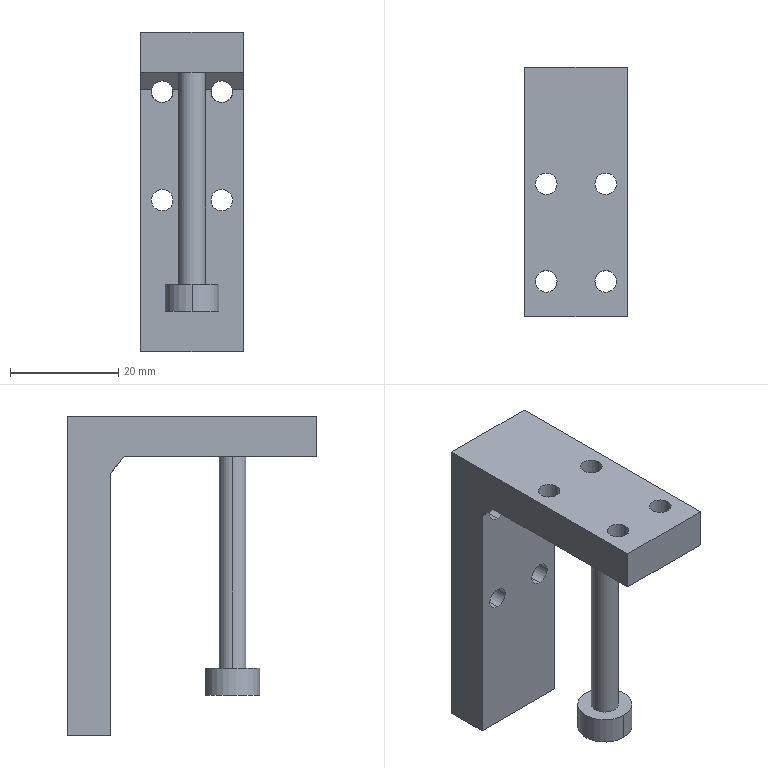Part | NX | 1 solid | 31 faces | box 19 x 46 x 59 mm | volume 14830 mm3 | cylinder 20 | plane 11 | commonest cylinder face diameters 4 x16 5 x2 10 x2
STEP:
#1=CARTESIAN_POINT('',(0.,5.,-51.5));
#2=VERTEX_POINT('',#1);
#3=CARTESIAN_POINT('',(0.,-5.,-51.5));
#4=VERTEX_POINT('',#3);
#5=CARTESIAN_POINT('',(0.,0.,-51.5));
#6=DIRECTION('',(0.,0.,-1.));
#7=DIRECTION('',(0.,1.,0.));
#8=AXIS2_PLACEMENT_3D('',#5,#6,#7);
#9=CIRCLE('',#8,5.);
#10=EDGE_CURVE('',#2,#4,#9,.T.);
#11=ORIENTED_EDGE('',*,*,#10,.F.);
#12=CARTESIAN_POINT('',(0.,5.,-46.5));
#13=VERTEX_POINT('',#12);
#14=CARTESIAN_POINT('',(0.,5.,-51.5));
#15=DIRECTION('',(0.,0.,1.));
#16=VECTOR('',#15,1000.);
#17=LINE('',#14,#16);
#18=EDGE_CURVE('',#2,#13,#17,.T.);
#19=ORIENTED_EDGE('',*,*,#18,.T.);
#20=CARTESIAN_POINT('',(0.,-5.,-46.5));
#21=VERTEX_POINT('',#20);
#22=CARTESIAN_POINT('',(0.,0.,-46.5));
#23=DIRECTION('',(0.,0.,-1.));
#24=DIRECTION('',(0.,1.,0.));
#25=AXIS2_PLACEMENT_3D('',#22,#23,#24);
#26=CIRCLE('',#25,5.);
#27=EDGE_CURVE('',#13,#21,#26,.T.);
#28=ORIENTED_EDGE('',*,*,#27,.T.);
#29=CARTESIAN_POINT('',(0.,-5.,-51.5));
#30=DIRECTION('',(0.,0.,1.));
#31=VECTOR('',#30,1000.);
#32=LINE('',#29,#31);
#33=EDGE_CURVE('',#4,#21,#32,.T.);
#34=ORIENTED_EDGE('',*,*,#33,.F.);
#35=EDGE_LOOP('',(#11,#19,#28,#34));
#36=FACE_BOUND('',#35,.T.);
#37=CARTESIAN_POINT('',(0.,0.,-51.5));
#38=DIRECTION('',(0.,0.,1.));
#39=DIRECTION('',(0.,-1.,0.));
#40=AXIS2_PLACEMENT_3D('',#37,#38,#39);
#41=CYLINDRICAL_SURFACE('',#40,5.);
#42=ADVANCED_FACE('',(#36),#41,.T.);
#43=CARTESIAN_POINT('',(5.5,22.5,-13.));
#44=VERTEX_POINT('',#43);
#45=CARTESIAN_POINT('',(3.564,22.5,-10.5));
#46=VERTEX_POINT('',#45);
#47=CARTESIAN_POINT('',(5.5,22.5,-11.));
#48=DIRECTION('',(0.,1.,0.));
#49=DIRECTION('',(0.,0.,1.));
#50=AXIS2_PLACEMENT_3D('',#47,#48,#49);
#51=CIRCLE('',#50,2.);
#52=EDGE_CURVE('',#44,#46,#51,.T.);
#53=ORIENTED_EDGE('',*,*,#52,.F.);
#54=CARTESIAN_POINT('',(5.5,30.5,-13.));
#55=VERTEX_POINT('',#54);
#56=CARTESIAN_POINT('',(5.5,-15.5,-13.));
#57=DIRECTION('',(0.,1.,0.));
#58=VECTOR('',#57,1000.);
#59=LINE('',#56,#58);
#60=EDGE_CURVE('',#44,#55,#59,.T.);
#61=ORIENTED_EDGE('',*,*,#60,.T.);
#62=CARTESIAN_POINT('',(5.5,30.5,-9.));
#63=VERTEX_POINT('',#62);
#64=CARTESIAN_POINT('',(5.5,30.5,-11.));
#65=DIRECTION('',(0.,1.,0.));
#66=DIRECTION('',(0.,0.,-1.));
#67=AXIS2_PLACEMENT_3D('',#64,#65,#66);
#68=CIRCLE('',#67,2.);
#69=EDGE_CURVE('',#55,#63,#68,.T.);
#70=ORIENTED_EDGE('',*,*,#69,.T.);
#71=CARTESIAN_POINT('',(5.5,21.241,-9.));
#72=VERTEX_POINT('',#71);
#73=CARTESIAN_POINT('',(5.5,-15.5,-9.));
#74=DIRECTION('',(0.,1.,0.));
#75=VECTOR('',#74,1000.);
#76=LINE('',#73,#75);
#77=EDGE_CURVE('',#72,#63,#76,.T.);
#78=ORIENTED_EDGE('',*,*,#77,.F.);
#79=CARTESIAN_POINT('',(3.564,22.5,-10.5));
#80=CARTESIAN_POINT('',(3.801,21.729,-9.581));
#81=CARTESIAN_POINT('',(4.551,21.241,-9.));
#82=CARTESIAN_POINT('',(5.5,21.241,-9.));
#83=(BOUNDED_CURVE()B_SPLINE_CURVE(3,(#79,#80,#81,#82),.UNSPECIFIED.,.F.,.F.)B_SPLINE_CURVE_WITH_KNOTS((4,4),(1.823,3.142),.UNSPECIFIED.)CURVE()GEOMETRIC_REPRESENTATION_ITEM()RATIONAL_B_SPLINE_CURVE((1.,0.8604,0.8604,1.))REPRESENTATION_ITEM(''));
#84=EDGE_CURVE('',#46,#72,#83,.T.);
#85=ORIENTED_EDGE('',*,*,#84,.F.);
#86=EDGE_LOOP('',(#53,#61,#70,#78,#85));
#87=FACE_BOUND('',#86,.T.);
#88=CARTESIAN_POINT('',(5.5,-15.5,-11.));
#89=DIRECTION('',(0.,1.,0.));
#90=DIRECTION('',(0.,0.,1.));
#91=AXIS2_PLACEMENT_3D('',#88,#89,#90);
#92=CYLINDRICAL_SURFACE('',#91,2.);
#93=ADVANCED_FACE('',(#87),#92,.F.);
#94=CARTESIAN_POINT('',(-5.5,22.5,-29.));
#95=VERTEX_POINT('',#94);
#96=CARTESIAN_POINT('',(-5.5,22.5,-33.));
#97=VERTEX_POINT('',#96);
#98=CARTESIAN_POINT('',(-5.5,22.5,-31.));
#99=DIRECTION('',(0.,1.,0.));
#100=DIRECTION('',(0.,0.,1.));
#101=AXIS2_PLACEMENT_3D('',#98,#99,#100);
#102=CIRCLE('',#101,2.);
#103=EDGE_CURVE('',#95,#97,#102,.T.);
#104=ORIENTED_EDGE('',*,*,#103,.F.);
#105=CARTESIAN_POINT('',(-5.5,30.5,-29.));
#106=VERTEX_POINT('',#105);
#107=CARTESIAN_POINT('',(-5.5,-15.5,-29.));
#108=DIRECTION('',(0.,1.,0.));
#109=VECTOR('',#108,1000.);
#110=LINE('',#107,#109);
#111=EDGE_CURVE('',#95,#106,#110,.T.);
#112=ORIENTED_EDGE('',*,*,#111,.T.);
#113=CARTESIAN_POINT('',(-5.5,30.5,-33.));
#114=VERTEX_POINT('',#113);
#115=CARTESIAN_POINT('',(-5.5,30.5,-31.));
#116=DIRECTION('',(0.,1.,0.));
#117=DIRECTION('',(0.,0.,1.));
#118=AXIS2_PLACEMENT_3D('',#115,#116,#117);
#119=CIRCLE('',#118,2.);
#120=EDGE_CURVE('',#106,#114,#119,.T.);
#121=ORIENTED_EDGE('',*,*,#120,.T.);
#122=CARTESIAN_POINT('',(-5.5,-15.5,-33.));
#123=DIRECTION('',(0.,1.,0.));
#124=VECTOR('',#123,1000.);
#125=LINE('',#122,#124);
#126=EDGE_CURVE('',#97,#114,#125,.T.);
#127=ORIENTED_EDGE('',*,*,#126,.F.);
#128=EDGE_LOOP('',(#104,#112,#121,#127));
#129=FACE_BOUND('',#128,.T.);
#130=CARTESIAN_POINT('',(-5.5,-15.5,-31.));
#131=DIRECTION('',(0.,1.,0.));
#132=DIRECTION('',(0.,0.,1.));
#133=AXIS2_PLACEMENT_3D('',#130,#131,#132);
#134=CYLINDRICAL_SURFACE('',#133,2.);
#135=ADVANCED_FACE('',(#129),#134,.F.);
#136=CARTESIAN_POINT('',(-5.5,22.5,-13.));
#137=VERTEX_POINT('',#136);
#138=CARTESIAN_POINT('',(-7.436,22.5,-10.5));
#139=VERTEX_POINT('',#138);
#140=CARTESIAN_POINT('',(-5.5,22.5,-11.));
#141=DIRECTION('',(0.,1.,0.));
#142=DIRECTION('',(0.,0.,1.));
#143=AXIS2_PLACEMENT_3D('',#140,#141,#142);
#144=CIRCLE('',#143,2.);
#145=EDGE_CURVE('',#137,#139,#144,.T.);
#146=ORIENTED_EDGE('',*,*,#145,.F.);
#147=CARTESIAN_POINT('',(-5.5,30.5,-13.));
#148=VERTEX_POINT('',#147);
#149=CARTESIAN_POINT('',(-5.5,-15.5,-13.));
#150=DIRECTION('',(0.,1.,0.));
#151=VECTOR('',#150,1000.);
#152=LINE('',#149,#151);
#153=EDGE_CURVE('',#137,#148,#152,.T.);
#154=ORIENTED_EDGE('',*,*,#153,.T.);
#155=CARTESIAN_POINT('',(-5.5,30.5,-9.));
#156=VERTEX_POINT('',#155);
#157=CARTESIAN_POINT('',(-5.5,30.5,-11.));
#158=DIRECTION('',(0.,1.,0.));
#159=DIRECTION('',(0.,0.,1.));
#160=AXIS2_PLACEMENT_3D('',#157,#158,#159);
#161=CIRCLE('',#160,2.);
#162=EDGE_CURVE('',#148,#156,#161,.T.);
#163=ORIENTED_EDGE('',*,*,#162,.T.);
#164=CARTESIAN_POINT('',(-5.5,21.241,-9.));
#165=VERTEX_POINT('',#164);
#166=CARTESIAN_POINT('',(-5.5,-15.5,-9.));
#167=DIRECTION('',(0.,1.,0.));
#168=VECTOR('',#167,1000.);
#169=LINE('',#166,#168);
#170=EDGE_CURVE('',#165,#156,#169,.T.);
#171=ORIENTED_EDGE('',*,*,#170,.F.);
#172=CARTESIAN_POINT('',(-7.436,22.5,-10.5));
#173=CARTESIAN_POINT('',(-7.199,21.729,-9.581));
#174=CARTESIAN_POINT('',(-6.449,21.241,-9.));
#175=CARTESIAN_POINT('',(-5.5,21.241,-9.));
#176=(BOUNDED_CURVE()B_SPLINE_CURVE(3,(#172,#173,#174,#175),.UNSPECIFIED.,.F.,.F.)B_SPLINE_CURVE_WITH_KNOTS((4,4),(1.823,3.142),.UNSPECIFIED.)CURVE()GEOMETRIC_REPRESENTATION_ITEM()RATIONAL_B_SPLINE_CURVE((1.,0.8604,0.8604,1.))REPRESENTATION_ITEM(''));
#177=EDGE_CURVE('',#139,#165,#176,.T.);
#178=ORIENTED_EDGE('',*,*,#177,.F.);
#179=EDGE_LOOP('',(#146,#154,#163,#171,#178));
#180=FACE_BOUND('',#179,.T.);
#181=CARTESIAN_POINT('',(-5.5,-15.5,-11.));
#182=DIRECTION('',(0.,1.,0.));
#183=DIRECTION('',(0.,0.,1.));
#184=AXIS2_PLACEMENT_3D('',#181,#182,#183);
#185=CYLINDRICAL_SURFACE('',#184,2.);
#186=ADVANCED_FACE('',(#180),#185,.F.);
#187=CARTESIAN_POINT('',(5.5,30.5,-33.));
#188=VERTEX_POINT('',#187);
#189=CARTESIAN_POINT('',(5.5,30.5,-29.));
#190=VERTEX_POINT('',#189);
#191=CARTESIAN_POINT('',(5.5,30.5,-31.));
#192=DIRECTION('',(0.,1.,0.));
#193=DIRECTION('',(0.,0.,-1.));
#194=AXIS2_PLACEMENT_3D('',#191,#192,#193);
#195=CIRCLE('',#194,2.);
#196=EDGE_CURVE('',#188,#190,#195,.T.);
#197=ORIENTED_EDGE('',*,*,#196,.T.);
#198=CARTESIAN_POINT('',(5.5,22.5,-29.));
#199=VERTEX_POINT('',#198);
#200=CARTESIAN_POINT('',(5.5,-15.5,-29.));
#201=DIRECTION('',(0.,1.,0.));
#202=VECTOR('',#201,1000.);
#203=LINE('',#200,#202);
#204=EDGE_CURVE('',#199,#190,#203,.T.);
#205=ORIENTED_EDGE('',*,*,#204,.F.);
#206=CARTESIAN_POINT('',(5.5,22.5,-33.));
#207=VERTEX_POINT('',#206);
#208=CARTESIAN_POINT('',(5.5,22.5,-31.));
#209=DIRECTION('',(0.,1.,0.));
#210=DIRECTION('',(0.,0.,1.));
#211=AXIS2_PLACEMENT_3D('',#208,#209,#210);
#212=CIRCLE('',#211,2.);
#213=EDGE_CURVE('',#207,#199,#212,.T.);
#214=ORIENTED_EDGE('',*,*,#213,.F.);
#215=CARTESIAN_POINT('',(5.5,-15.5,-33.));
#216=DIRECTION('',(0.,1.,0.));
#217=VECTOR('',#216,1000.);
#218=LINE('',#215,#217);
#219=EDGE_CURVE('',#207,#188,#218,.T.);
#220=ORIENTED_EDGE('',*,*,#219,.T.);
#221=EDGE_LOOP('',(#197,#205,#214,#220));
#222=FACE_BOUND('',#221,.T.);
#223=CARTESIAN_POINT('',(5.5,-15.5,-31.));
#224=DIRECTION('',(0.,1.,0.));
#225=DIRECTION('',(0.,0.,1.));
#226=AXIS2_PLACEMENT_3D('',#223,#224,#225);
#227=CYLINDRICAL_SURFACE('',#226,2.);
#228=ADVANCED_FACE('',(#222),#227,.F.);
#229=CARTESIAN_POINT('',(3.5,-9.,-7.5));
#230=VERTEX_POINT('',#229);
#231=CARTESIAN_POINT('',(7.5,-9.,-7.5));
#232=VERTEX_POINT('',#231);
#233=CARTESIAN_POINT('',(5.5,-9.,-7.5));
#234=DIRECTION('',(0.,0.,1.));
#235=DIRECTION('',(0.,-1.,0.));
#236=AXIS2_PLACEMENT_3D('',#233,#234,#235);
#237=CIRCLE('',#236,2.);
#238=EDGE_CURVE('',#230,#232,#237,.T.);
#239=ORIENTED_EDGE('',*,*,#238,.F.);
#240=CARTESIAN_POINT('',(3.5,-9.,0.));
#241=VERTEX_POINT('',#240);
#242=CARTESIAN_POINT('',(3.5,-9.,-59.));
#243=DIRECTION('',(0.,0.,1.));
#244=VECTOR('',#243,1000.);
#245=LINE('',#242,#244);
#246=EDGE_CURVE('',#230,#241,#245,.T.);
#247=ORIENTED_EDGE('',*,*,#246,.T.);
#248=CARTESIAN_POINT('',(7.5,-9.,0.));
#249=VERTEX_POINT('',#248);
#250=CARTESIAN_POINT('',(5.5,-9.,0.));
#251=DIRECTION('',(0.,0.,1.));
#252=DIRECTION('',(-1.,0.,0.));
#253=AXIS2_PLACEMENT_3D('',#250,#251,#252);
#254=CIRCLE('',#253,2.);
#255=EDGE_CURVE('',#241,#249,#254,.T.);
#256=ORIENTED_EDGE('',*,*,#255,.T.);
#257=CARTESIAN_POINT('',(7.5,-9.,-59.));
#258=DIRECTION('',(0.,0.,1.));
#259=VECTOR('',#258,1000.);
#260=LINE('',#257,#259);
#261=EDGE_CURVE('',#232,#249,#260,.T.);
#262=ORIENTED_EDGE('',*,*,#261,.F.);
#263=EDGE_LOOP('',(#239,#247,#256,#262));
#264=FACE_BOUND('',#263,.T.);
#265=CARTESIAN_POINT('',(5.5,-9.,-59.));
#266=DIRECTION('',(0.,0.,1.));
#267=DIRECTION('',(1.,0.,0.));
#268=AXIS2_PLACEMENT_3D('',#265,#266,#267);
#269=CYLINDRICAL_SURFACE('',#268,2.);
#270=ADVANCED_FACE('',(#264),#269,.F.);
#271=CARTESIAN_POINT('',(-3.5,-9.,0.));
#272=VERTEX_POINT('',#271);
#273=CARTESIAN_POINT('',(-7.5,-9.,0.));
#274=VERTEX_POINT('',#273);
#275=CARTESIAN_POINT('',(-5.5,-9.,0.));
#276=DIRECTION('',(0.,0.,1.));
#277=DIRECTION('',(1.,0.,0.));
#278=AXIS2_PLACEMENT_3D('',#275,#276,#277);
#279=CIRCLE('',#278,2.);
#280=EDGE_CURVE('',#272,#274,#279,.T.);
#281=ORIENTED_EDGE('',*,*,#280,.T.);
#282=CARTESIAN_POINT('',(-7.5,-9.,-7.5));
#283=VERTEX_POINT('',#282);
#284=CARTESIAN_POINT('',(-7.5,-9.,-59.));
#285=DIRECTION('',(0.,0.,1.));
#286=VECTOR('',#285,1000.);
#287=LINE('',#284,#286);
#288=EDGE_CURVE('',#283,#274,#287,.T.);
#289=ORIENTED_EDGE('',*,*,#288,.F.);
#290=CARTESIAN_POINT('',(-3.5,-9.,-7.5));
#291=VERTEX_POINT('',#290);
#292=CARTESIAN_POINT('',(-5.5,-9.,-7.5));
#293=DIRECTION('',(0.,0.,1.));
#294=DIRECTION('',(0.,-1.,0.));
#295=AXIS2_PLACEMENT_3D('',#292,#293,#294);
#296=CIRCLE('',#295,2.);
#297=EDGE_CURVE('',#291,#283,#296,.T.);
#298=ORIENTED_EDGE('',*,*,#297,.F.);
#299=CARTESIAN_POINT('',(-3.5,-9.,-59.));
#300=DIRECTION('',(0.,0.,1.));
#301=VECTOR('',#300,1000.);
#302=LINE('',#299,#301);
#303=EDGE_CURVE('',#291,#272,#302,.T.);
#304=ORIENTED_EDGE('',*,*,#303,.T.);
#305=EDGE_LOOP('',(#281,#289,#298,#304));
#306=FACE_BOUND('',#305,.T.);
#307=CARTESIAN_POINT('',(-5.5,-9.,-59.));
#308=DIRECTION('',(0.,0.,1.));
#309=DIRECTION('',(1.,0.,0.));
#310=AXIS2_PLACEMENT_3D('',#307,#308,#309);
#311=CYLINDRICAL_SURFACE('',#310,2.);
#312=ADVANCED_FACE('',(#306),#311,.F.);
#313=CARTESIAN_POINT('',(-3.5,9.,-7.5));
#314=VERTEX_POINT('',#313);
#315=CARTESIAN_POINT('',(-7.5,9.,-7.5));
#316=VERTEX_POINT('',#315);
#317=CARTESIAN_POINT('',(-5.5,9.,-7.5));
#318=DIRECTION('',(0.,0.,1.));
#319=DIRECTION('',(0.,-1.,0.));
#320=AXIS2_PLACEMENT_3D('',#317,#318,#319);
#321=CIRCLE('',#320,2.);
#322=EDGE_CURVE('',#314,#316,#321,.T.);
#323=ORIENTED_EDGE('',*,*,#322,.F.);
#324=CARTESIAN_POINT('',(-3.5,9.,0.));
#325=VERTEX_POINT('',#324);
#326=CARTESIAN_POINT('',(-3.5,9.,-59.));
#327=DIRECTION('',(0.,0.,1.));
#328=VECTOR('',#327,1000.);
#329=LINE('',#326,#328);
#330=EDGE_CURVE('',#314,#325,#329,.T.);
#331=ORIENTED_EDGE('',*,*,#330,.T.);
#332=CARTESIAN_POINT('',(-7.5,9.,0.));
#333=VERTEX_POINT('',#332);
#334=CARTESIAN_POINT('',(-5.5,9.,0.));
#335=DIRECTION('',(0.,0.,1.));
#336=DIRECTION('',(-1.,0.,0.));
#337=AXIS2_PLACEMENT_3D('',#334,#335,#336);
#338=CIRCLE('',#337,2.);
#339=EDGE_CURVE('',#325,#333,#338,.T.);
#340=ORIENTED_EDGE('',*,*,#339,.T.);
#341=CARTESIAN_POINT('',(-7.5,9.,-59.));
#342=DIRECTION('',(0.,0.,1.));
#343=VECTOR('',#342,1000.);
#344=LINE('',#341,#343);
#345=EDGE_CURVE('',#316,#333,#344,.T.);
#346=ORIENTED_EDGE('',*,*,#345,.F.);
#347=EDGE_LOOP('',(#323,#331,#340,#346));
#348=FACE_BOUND('',#347,.T.);
#349=CARTESIAN_POINT('',(-5.5,9.,-59.));
#350=DIRECTION('',(0.,0.,1.));
#351=DIRECTION('',(1.,0.,0.));
#352=AXIS2_PLACEMENT_3D('',#349,#350,#351);
#353=CYLINDRICAL_SURFACE('',#352,2.);
#354=ADVANCED_FACE('',(#348),#353,.F.);
#355=CARTESIAN_POINT('',(7.5,9.,-7.5));
#356=VERTEX_POINT('',#355);
#357=CARTESIAN_POINT('',(3.5,9.,-7.5));
#358=VERTEX_POINT('',#357);
#359=CARTESIAN_POINT('',(5.5,9.,-7.5));
#360=DIRECTION('',(0.,0.,1.));
#361=DIRECTION('',(0.,-1.,0.));
#362=AXIS2_PLACEMENT_3D('',#359,#360,#361);
#363=CIRCLE('',#362,2.);
#364=EDGE_CURVE('',#356,#358,#363,.T.);
#365=ORIENTED_EDGE('',*,*,#364,.F.);
#366=CARTESIAN_POINT('',(7.5,9.,0.));
#367=VERTEX_POINT('',#366);
#368=CARTESIAN_POINT('',(7.5,9.,-59.));
#369=DIRECTION('',(0.,0.,1.));
#370=VECTOR('',#369,1000.);
#371=LINE('',#368,#370);
#372=EDGE_CURVE('',#356,#367,#371,.T.);
#373=ORIENTED_EDGE('',*,*,#372,.T.);
#374=CARTESIAN_POINT('',(3.5,9.,0.));
#375=VERTEX_POINT('',#374);
#376=CARTESIAN_POINT('',(5.5,9.,0.));
#377=DIRECTION('',(0.,0.,1.));
#378=DIRECTION('',(1.,0.,0.));
#379=AXIS2_PLACEMENT_3D('',#376,#377,#378);
#380=CIRCLE('',#379,2.);
#381=EDGE_CURVE('',#367,#375,#380,.T.);
#382=ORIENTED_EDGE('',*,*,#381,.T.);
#383=CARTESIAN_POINT('',(3.5,9.,-59.));
#384=DIRECTION('',(0.,0.,1.));
#385=VECTOR('',#384,1000.);
#386=LINE('',#383,#385);
#387=EDGE_CURVE('',#358,#375,#386,.T.);
#388=ORIENTED_EDGE('',*,*,#387,.F.);
#389=EDGE_LOOP('',(#365,#373,#382,#388));
#390=FACE_BOUND('',#389,.T.);
#391=CARTESIAN_POINT('',(5.5,9.,-59.));
#392=DIRECTION('',(0.,0.,1.));
#393=DIRECTION('',(1.,0.,0.));
#394=AXIS2_PLACEMENT_3D('',#391,#392,#393);
#395=CYLINDRICAL_SURFACE('',#394,2.);
#396=ADVANCED_FACE('',(#390),#395,.F.);
#397=CARTESIAN_POINT('',(2.5,0.,-46.5));
#398=VERTEX_POINT('',#397);
#399=CARTESIAN_POINT('',(-2.5,0.,-46.5));
#400=VERTEX_POINT('',#399);
#401=CARTESIAN_POINT('',(0.,0.,-46.5));
#402=DIRECTION('',(0.,0.,-1.));
#403=DIRECTION('',(0.,1.,0.));
#404=AXIS2_PLACEMENT_3D('',#401,#402,#403);
#405=CIRCLE('',#404,2.5);
#406=EDGE_CURVE('',#398,#400,#405,.T.);
#407=ORIENTED_EDGE('',*,*,#406,.F.);
#408=CARTESIAN_POINT('',(2.5,0.,-7.5));
#409=VERTEX_POINT('',#408);
#410=CARTESIAN_POINT('',(2.5,0.,-49.));
#411=DIRECTION('',(0.,0.,1.));
#412=VECTOR('',#411,1000.);
#413=LINE('',#410,#412);
#414=EDGE_CURVE('',#398,#409,#413,.T.);
#415=ORIENTED_EDGE('',*,*,#414,.T.);
#416=CARTESIAN_POINT('',(-2.5,0.,-7.5));
#417=VERTEX_POINT('',#416);
#418=CARTESIAN_POINT('',(0.,0.,-7.5));
#419=DIRECTION('',(0.,0.,-1.));
#420=DIRECTION('',(0.,-1.,0.));
#421=AXIS2_PLACEMENT_3D('',#418,#419,#420);
#422=CIRCLE('',#421,2.5);
#423=EDGE_CURVE('',#409,#417,#422,.T.);
#424=ORIENTED_EDGE('',*,*,#423,.T.);
#425=CARTESIAN_POINT('',(-2.5,0.,-49.));
#426=DIRECTION('',(0.,0.,1.));
#427=VECTOR('',#426,1000.);
#428=LINE('',#425,#427);
#429=EDGE_CURVE('',#400,#417,#428,.T.);
#430=ORIENTED_EDGE('',*,*,#429,.F.);
#431=EDGE_LOOP('',(#407,#415,#424,#430));
#432=FACE_BOUND('',#431,.T.);
#433=CARTESIAN_POINT('',(0.,0.,-49.));
#434=DIRECTION('',(0.,0.,1.));
#435=DIRECTION('',(1.,0.,0.));
#436=AXIS2_PLACEMENT_3D('',#433,#434,#435);
#437=CYLINDRICAL_SURFACE('',#436,2.5);
#438=ADVANCED_FACE('',(#432),#437,.T.);
#439=CARTESIAN_POINT('',(0.,0.,-46.5));
#440=DIRECTION('',(0.,0.,-1.));
#441=DIRECTION('',(0.,1.,0.));
#442=AXIS2_PLACEMENT_3D('',#439,#440,#441);
#443=CIRCLE('',#442,5.);
#444=EDGE_CURVE('',#21,#13,#443,.T.);
#445=ORIENTED_EDGE('',*,*,#444,.F.);
#446=ORIENTED_EDGE('',*,*,#27,.F.);
#447=EDGE_LOOP('',(#445,#446));
#448=FACE_BOUND('',#447,.T.);
#449=ORIENTED_EDGE('',*,*,#406,.T.);
#450=CARTESIAN_POINT('',(0.,0.,-46.5));
#451=DIRECTION('',(0.,0.,-1.));
#452=DIRECTION('',(0.,1.,0.));
#453=AXIS2_PLACEMENT_3D('',#450,#451,#452);
#454=CIRCLE('',#453,2.5);
#455=EDGE_CURVE('',#400,#398,#454,.T.);
#456=ORIENTED_EDGE('',*,*,#455,.T.);
#457=EDGE_LOOP('',(#449,#456));
#458=FACE_BOUND('',#457,.T.);
#459=CARTESIAN_POINT('',(0.,0.,-46.5));
#460=DIRECTION('',(0.,0.,-1.));
#461=DIRECTION('',(-1.,0.,0.));
#462=AXIS2_PLACEMENT_3D('',#459,#460,#461);
#463=PLANE('',#462);
#464=ADVANCED_FACE('',(#448,#458),#463,.F.);
#465=CARTESIAN_POINT('',(-9.5,-15.5,-7.5));
#466=VERTEX_POINT('',#465);
#467=CARTESIAN_POINT('',(-9.5,19.983,-7.5));
#468=VERTEX_POINT('',#467);
#469=CARTESIAN_POINT('',(-9.5,19.983,-7.5));
#470=DIRECTION('',(0.,1.,0.));
#471=VECTOR('',#470,1000.);
#472=LINE('',#469,#471);
#473=EDGE_CURVE('',#466,#468,#472,.T.);
#474=ORIENTED_EDGE('',*,*,#473,.T.);
#475=CARTESIAN_POINT('',(9.5,19.983,-7.5));
#476=VERTEX_POINT('',#475);
#477=CARTESIAN_POINT('',(9.5,19.983,-7.5));
#478=DIRECTION('',(-1.,0.,0.));
#479=VECTOR('',#478,1000.);
#480=LINE('',#477,#479);
#481=EDGE_CURVE('',#476,#468,#480,.T.);
#482=ORIENTED_EDGE('',*,*,#481,.F.);
#483=CARTESIAN_POINT('',(9.5,-15.5,-7.5));
#484=VERTEX_POINT('',#483);
#485=CARTESIAN_POINT('',(9.5,19.983,-7.5));
#486=DIRECTION('',(0.,1.,0.));
#487=VECTOR('',#486,1000.);
#488=LINE('',#485,#487);
#489=EDGE_CURVE('',#484,#476,#488,.T.);
#490=ORIENTED_EDGE('',*,*,#489,.F.);
#491=CARTESIAN_POINT('',(9.5,-15.5,-7.5));
#492=DIRECTION('',(-1.,0.,0.));
#493=VECTOR('',#492,1000.);
#494=LINE('',#491,#493);
#495=EDGE_CURVE('',#484,#466,#494,.T.);
#496=ORIENTED_EDGE('',*,*,#495,.T.);
#497=EDGE_LOOP('',(#474,#482,#490,#496));
#498=FACE_BOUND('',#497,.T.);
#499=ORIENTED_EDGE('',*,*,#364,.T.);
#500=CARTESIAN_POINT('',(5.5,9.,-7.5));
#501=DIRECTION('',(0.,0.,1.));
#502=DIRECTION('',(0.,-1.,0.));
#503=AXIS2_PLACEMENT_3D('',#500,#501,#502);
#504=CIRCLE('',#503,2.);
#505=EDGE_CURVE('',#358,#356,#504,.T.);
#506=ORIENTED_EDGE('',*,*,#505,.T.);
#507=EDGE_LOOP('',(#499,#506));
#508=FACE_BOUND('',#507,.T.);
#509=ORIENTED_EDGE('',*,*,#322,.T.);
#510=CARTESIAN_POINT('',(-5.5,9.,-7.5));
#511=DIRECTION('',(0.,0.,1.));
#512=DIRECTION('',(0.,-1.,0.));
#513=AXIS2_PLACEMENT_3D('',#510,#511,#512);
#514=CIRCLE('',#513,2.);
#515=EDGE_CURVE('',#316,#314,#514,.T.);
#516=ORIENTED_EDGE('',*,*,#515,.T.);
#517=EDGE_LOOP('',(#509,#516));
#518=FACE_BOUND('',#517,.T.);
#519=ORIENTED_EDGE('',*,*,#297,.T.);
#520=CARTESIAN_POINT('',(-5.5,-9.,-7.5));
#521=DIRECTION('',(0.,0.,1.));
#522=DIRECTION('',(0.,-1.,0.));
#523=AXIS2_PLACEMENT_3D('',#520,#521,#522);
#524=CIRCLE('',#523,2.);
#525=EDGE_CURVE('',#283,#291,#524,.T.);
#526=ORIENTED_EDGE('',*,*,#525,.T.);
#527=EDGE_LOOP('',(#519,#526));
#528=FACE_BOUND('',#527,.T.);
#529=ORIENTED_EDGE('',*,*,#238,.T.);
#530=CARTESIAN_POINT('',(5.5,-9.,-7.5));
#531=DIRECTION('',(0.,0.,1.));
#532=DIRECTION('',(0.,-1.,0.));
#533=AXIS2_PLACEMENT_3D('',#530,#531,#532);
#534=CIRCLE('',#533,2.);
#535=EDGE_CURVE('',#232,#230,#534,.T.);
#536=ORIENTED_EDGE('',*,*,#535,.T.);
#537=EDGE_LOOP('',(#529,#536));
#538=FACE_BOUND('',#537,.T.);
#539=ORIENTED_EDGE('',*,*,#423,.F.);
#540=CARTESIAN_POINT('',(0.,0.,-7.5));
#541=DIRECTION('',(0.,0.,-1.));
#542=DIRECTION('',(0.,-1.,0.));
#543=AXIS2_PLACEMENT_3D('',#540,#541,#542);
#544=CIRCLE('',#543,2.5);
#545=EDGE_CURVE('',#417,#409,#544,.T.);
#546=ORIENTED_EDGE('',*,*,#545,.F.);
#547=EDGE_LOOP('',(#539,#546));
#548=FACE_BOUND('',#547,.T.);
#549=CARTESIAN_POINT('',(9.5,19.983,-7.5));
#550=DIRECTION('',(0.,0.,1.));
#551=DIRECTION('',(0.,-1.,0.));
#552=AXIS2_PLACEMENT_3D('',#549,#550,#551);
#553=PLANE('',#552);
#554=ADVANCED_FACE('',(#498,#508,#518,#528,#538,#548),#553,.F.);
#555=CARTESIAN_POINT('',(-9.5,-15.5,0.));
#556=VERTEX_POINT('',#555);
#557=CARTESIAN_POINT('',(-9.5,-15.5,-7.5));
#558=DIRECTION('',(0.,0.,-1.));
#559=VECTOR('',#558,1000.);
#560=LINE('',#557,#559);
#561=EDGE_CURVE('',#556,#466,#560,.T.);
#562=ORIENTED_EDGE('',*,*,#561,.T.);
#563=ORIENTED_EDGE('',*,*,#495,.F.);
#564=CARTESIAN_POINT('',(9.5,-15.5,0.));
#565=VERTEX_POINT('',#564);
#566=CARTESIAN_POINT('',(9.5,-15.5,-7.5));
#567=DIRECTION('',(0.,0.,-1.));
#568=VECTOR('',#567,1000.);
#569=LINE('',#566,#568);
#570=EDGE_CURVE('',#565,#484,#569,.T.);
#571=ORIENTED_EDGE('',*,*,#570,.F.);
#572=CARTESIAN_POINT('',(9.5,-15.5,0.));
#573=DIRECTION('',(-1.,0.,0.));
#574=VECTOR('',#573,1000.);
#575=LINE('',#572,#574);
#576=EDGE_CURVE('',#565,#556,#575,.T.);
#577=ORIENTED_EDGE('',*,*,#576,.T.);
#578=EDGE_LOOP('',(#562,#563,#571,#577));
#579=FACE_BOUND('',#578,.T.);
#580=CARTESIAN_POINT('',(9.5,-15.5,-7.5));
#581=DIRECTION('',(0.,1.,0.));
#582=DIRECTION('',(1.,0.,0.));
#583=AXIS2_PLACEMENT_3D('',#580,#581,#582);
#584=PLANE('',#583);
#585=ADVANCED_FACE('',(#579),#584,.F.);
#586=CARTESIAN_POINT('',(-3.564,22.5,-10.5));
#587=VERTEX_POINT('',#586);
#588=CARTESIAN_POINT('',(9.5,22.5,-10.5));
#589=DIRECTION('',(-1.,0.,0.));
#590=VECTOR('',#589,1000.);
#591=LINE('',#588,#590);
#592=EDGE_CURVE('',#46,#587,#591,.T.);
#593=ORIENTED_EDGE('',*,*,#592,.F.);
#594=ORIENTED_EDGE('',*,*,#84,.T.);
#595=CARTESIAN_POINT('',(7.436,22.5,-10.5));
#596=VERTEX_POINT('',#595);
#597=CARTESIAN_POINT('',(5.5,21.241,-9.));
#598=CARTESIAN_POINT('',(6.449,21.241,-9.));
#599=CARTESIAN_POINT('',(7.199,21.729,-9.581));
#600=CARTESIAN_POINT('',(7.436,22.5,-10.5));
#601=(BOUNDED_CURVE()B_SPLINE_CURVE(3,(#597,#598,#599,#600),.UNSPECIFIED.,.F.,.F.)B_SPLINE_CURVE_WITH_KNOTS((4,4),(3.142,4.46),.UNSPECIFIED.)CURVE()GEOMETRIC_REPRESENTATION_ITEM()RATIONAL_B_SPLINE_CURVE((1.,0.8604,0.8604,1.))REPRESENTATION_ITEM(''));
#602=EDGE_CURVE('',#72,#596,#601,.T.);
#603=ORIENTED_EDGE('',*,*,#602,.T.);
#604=CARTESIAN_POINT('',(9.5,22.5,-10.5));
#605=VERTEX_POINT('',#604);
#606=CARTESIAN_POINT('',(9.5,22.5,-10.5));
#607=DIRECTION('',(-1.,0.,0.));
#608=VECTOR('',#607,1000.);
#609=LINE('',#606,#608);
#610=EDGE_CURVE('',#605,#596,#609,.T.);
#611=ORIENTED_EDGE('',*,*,#610,.F.);
#612=CARTESIAN_POINT('',(9.5,22.5,-10.5));
#613=DIRECTION('',(0.,0.6428,-0.766));
#614=VECTOR('',#613,1000.);
#615=LINE('',#612,#614);
#616=EDGE_CURVE('',#476,#605,#615,.T.);
#617=ORIENTED_EDGE('',*,*,#616,.F.);
#618=ORIENTED_EDGE('',*,*,#481,.T.);
#619=CARTESIAN_POINT('',(-9.5,22.5,-10.5));
#620=VERTEX_POINT('',#619);
#621=CARTESIAN_POINT('',(-9.5,22.5,-10.5));
#622=DIRECTION('',(0.,0.6428,-0.766));
#623=VECTOR('',#622,1000.);
#624=LINE('',#621,#623);
#625=EDGE_CURVE('',#468,#620,#624,.T.);
#626=ORIENTED_EDGE('',*,*,#625,.T.);
#627=CARTESIAN_POINT('',(9.5,22.5,-10.5));
#628=DIRECTION('',(-1.,0.,0.));
#629=VECTOR('',#628,1000.);
#630=LINE('',#627,#629);
#631=EDGE_CURVE('',#139,#620,#630,.T.);
#632=ORIENTED_EDGE('',*,*,#631,.F.);
#633=ORIENTED_EDGE('',*,*,#177,.T.);
#634=CARTESIAN_POINT('',(-5.5,21.241,-9.));
#635=CARTESIAN_POINT('',(-4.551,21.241,-9.));
#636=CARTESIAN_POINT('',(-3.801,21.729,-9.581));
#637=CARTESIAN_POINT('',(-3.564,22.5,-10.5));
#638=(BOUNDED_CURVE()B_SPLINE_CURVE(3,(#634,#635,#636,#637),.UNSPECIFIED.,.F.,.F.)B_SPLINE_CURVE_WITH_KNOTS((4,4),(3.142,4.46),.UNSPECIFIED.)CURVE()GEOMETRIC_REPRESENTATION_ITEM()RATIONAL_B_SPLINE_CURVE((1.,0.8604,0.8604,1.))REPRESENTATION_ITEM(''));
#639=EDGE_CURVE('',#165,#587,#638,.T.);
#640=ORIENTED_EDGE('',*,*,#639,.T.);
#641=EDGE_LOOP('',(#593,#594,#603,#611,#617,#618,#626,#632,#633,#640));
#642=FACE_BOUND('',#641,.T.);
#643=CARTESIAN_POINT('',(9.5,22.5,-10.5));
#644=DIRECTION('',(0.,0.766,0.6428));
#645=DIRECTION('',(1.,0.,0.));
#646=AXIS2_PLACEMENT_3D('',#643,#644,#645);
#647=PLANE('',#646);
#648=ADVANCED_FACE('',(#642),#647,.F.);
#649=ORIENTED_EDGE('',*,*,#610,.T.);
#650=CARTESIAN_POINT('',(5.5,22.5,-11.));
#651=DIRECTION('',(0.,1.,0.));
#652=DIRECTION('',(0.,0.,1.));
#653=AXIS2_PLACEMENT_3D('',#650,#651,#652);
#654=CIRCLE('',#653,2.);
#655=EDGE_CURVE('',#596,#44,#654,.T.);
#656=ORIENTED_EDGE('',*,*,#655,.T.);
#657=ORIENTED_EDGE('',*,*,#52,.T.);
#658=ORIENTED_EDGE('',*,*,#592,.T.);
#659=CARTESIAN_POINT('',(-5.5,22.5,-11.));
#660=DIRECTION('',(0.,1.,0.));
#661=DIRECTION('',(0.,0.,1.));
#662=AXIS2_PLACEMENT_3D('',#659,#660,#661);
#663=CIRCLE('',#662,2.);
#664=EDGE_CURVE('',#587,#137,#663,.T.);
#665=ORIENTED_EDGE('',*,*,#664,.T.);
#666=ORIENTED_EDGE('',*,*,#145,.T.);
#667=ORIENTED_EDGE('',*,*,#631,.T.);
#668=CARTESIAN_POINT('',(-9.5,22.5,-59.));
#669=VERTEX_POINT('',#668);
#670=CARTESIAN_POINT('',(-9.5,22.5,-59.));
#671=DIRECTION('',(0.,0.,-1.));
#672=VECTOR('',#671,1000.);
#673=LINE('',#670,#672);
#674=EDGE_CURVE('',#620,#669,#673,.T.);
#675=ORIENTED_EDGE('',*,*,#674,.T.);
#676=CARTESIAN_POINT('',(9.5,22.5,-59.));
#677=VERTEX_POINT('',#676);
#678=CARTESIAN_POINT('',(9.5,22.5,-59.));
#679=DIRECTION('',(-1.,0.,0.));
#680=VECTOR('',#679,1000.);
#681=LINE('',#678,#680);
#682=EDGE_CURVE('',#677,#669,#681,.T.);
#683=ORIENTED_EDGE('',*,*,#682,.F.);
#684=CARTESIAN_POINT('',(9.5,22.5,-59.));
#685=DIRECTION('',(0.,0.,-1.));
#686=VECTOR('',#685,1000.);
#687=LINE('',#684,#686);
#688=EDGE_CURVE('',#605,#677,#687,.T.);
#689=ORIENTED_EDGE('',*,*,#688,.F.);
#690=EDGE_LOOP('',(#649,#656,#657,#658,#665,#666,#667,#675,#683,#689));
#691=FACE_BOUND('',#690,.T.);
#692=ORIENTED_EDGE('',*,*,#103,.T.);
#693=CARTESIAN_POINT('',(-5.5,22.5,-31.));
#694=DIRECTION('',(0.,1.,0.));
#695=DIRECTION('',(0.,0.,1.));
#696=AXIS2_PLACEMENT_3D('',#693,#694,#695);
#697=CIRCLE('',#696,2.);
#698=EDGE_CURVE('',#97,#95,#697,.T.);
#699=ORIENTED_EDGE('',*,*,#698,.T.);
#700=EDGE_LOOP('',(#692,#699));
#701=FACE_BOUND('',#700,.T.);
#702=ORIENTED_EDGE('',*,*,#213,.T.);
#703=CARTESIAN_POINT('',(5.5,22.5,-31.));
#704=DIRECTION('',(0.,1.,0.));
#705=DIRECTION('',(0.,0.,1.));
#706=AXIS2_PLACEMENT_3D('',#703,#704,#705);
#707=CIRCLE('',#706,2.);
#708=EDGE_CURVE('',#199,#207,#707,.T.);
#709=ORIENTED_EDGE('',*,*,#708,.T.);
#710=EDGE_LOOP('',(#702,#709));
#711=FACE_BOUND('',#710,.T.);
#712=CARTESIAN_POINT('',(9.5,22.5,-59.));
#713=DIRECTION('',(0.,1.,0.));
#714=DIRECTION('',(0.,0.,-1.));
#715=AXIS2_PLACEMENT_3D('',#712,#713,#714);
#716=PLANE('',#715);
#717=ADVANCED_FACE('',(#691,#701,#711),#716,.F.);
#718=CARTESIAN_POINT('',(-9.5,30.5,-59.));
#719=VERTEX_POINT('',#718);
#720=CARTESIAN_POINT('',(-9.5,30.5,-59.));
#721=DIRECTION('',(0.,1.,0.));
#722=VECTOR('',#721,1000.);
#723=LINE('',#720,#722);
#724=EDGE_CURVE('',#669,#719,#723,.T.);
#725=ORIENTED_EDGE('',*,*,#724,.T.);
#726=CARTESIAN_POINT('',(9.5,30.5,-59.));
#727=VERTEX_POINT('',#726);
#728=CARTESIAN_POINT('',(9.5,30.5,-59.));
#729=DIRECTION('',(-1.,0.,0.));
#730=VECTOR('',#729,1000.);
#731=LINE('',#728,#730);
#732=EDGE_CURVE('',#727,#719,#731,.T.);
#733=ORIENTED_EDGE('',*,*,#732,.F.);
#734=CARTESIAN_POINT('',(9.5,30.5,-59.));
#735=DIRECTION('',(0.,1.,0.));
#736=VECTOR('',#735,1000.);
#737=LINE('',#734,#736);
#738=EDGE_CURVE('',#677,#727,#737,.T.);
#739=ORIENTED_EDGE('',*,*,#738,.F.);
#740=ORIENTED_EDGE('',*,*,#682,.T.);
#741=EDGE_LOOP('',(#725,#733,#739,#740));
#742=FACE_BOUND('',#741,.T.);
#743=CARTESIAN_POINT('',(9.5,30.5,-59.));
#744=DIRECTION('',(0.,0.,1.));
#745=DIRECTION('',(1.,0.,0.));
#746=AXIS2_PLACEMENT_3D('',#743,#744,#745);
#747=PLANE('',#746);
#748=ADVANCED_FACE('',(#742),#747,.F.);
#749=CARTESIAN_POINT('',(-9.5,30.5,0.));
#750=VERTEX_POINT('',#749);
#751=CARTESIAN_POINT('',(-9.5,30.5,0.));
#752=DIRECTION('',(0.,0.,1.));
#753=VECTOR('',#752,1000.);
#754=LINE('',#751,#753);
#755=EDGE_CURVE('',#719,#750,#754,.T.);
#756=ORIENTED_EDGE('',*,*,#755,.T.);
#757=CARTESIAN_POINT('',(9.5,30.5,0.));
#758=VERTEX_POINT('',#757);
#759=CARTESIAN_POINT('',(9.5,30.5,0.));
#760=DIRECTION('',(-1.,0.,0.));
#761=VECTOR('',#760,1000.);
#762=LINE('',#759,#761);
#763=EDGE_CURVE('',#758,#750,#762,.T.);
#764=ORIENTED_EDGE('',*,*,#763,.F.);
#765=CARTESIAN_POINT('',(9.5,30.5,0.));
#766=DIRECTION('',(0.,0.,1.));
#767=VECTOR('',#766,1000.);
#768=LINE('',#765,#767);
#769=EDGE_CURVE('',#727,#758,#768,.T.);
#770=ORIENTED_EDGE('',*,*,#769,.F.);
#771=ORIENTED_EDGE('',*,*,#732,.T.);
#772=EDGE_LOOP('',(#756,#764,#770,#771));
#773=FACE_BOUND('',#772,.T.);
#774=CARTESIAN_POINT('',(5.5,30.5,-11.));
#775=DIRECTION('',(0.,1.,0.));
#776=DIRECTION('',(0.,0.,-1.));
#777=AXIS2_PLACEMENT_3D('',#774,#775,#776);
#778=CIRCLE('',#777,2.);
#779=EDGE_CURVE('',#63,#55,#778,.T.);
#780=ORIENTED_EDGE('',*,*,#779,.F.);
#781=ORIENTED_EDGE('',*,*,#69,.F.);
#782=EDGE_LOOP('',(#780,#781));
#783=FACE_BOUND('',#782,.T.);
#784=CARTESIAN_POINT('',(-5.5,30.5,-31.));
#785=DIRECTION('',(0.,1.,0.));
#786=DIRECTION('',(0.,0.,1.));
#787=AXIS2_PLACEMENT_3D('',#784,#785,#786);
#788=CIRCLE('',#787,2.);
#789=EDGE_CURVE('',#114,#106,#788,.T.);
#790=ORIENTED_EDGE('',*,*,#789,.F.);
#791=ORIENTED_EDGE('',*,*,#120,.F.);
#792=EDGE_LOOP('',(#790,#791));
#793=FACE_BOUND('',#792,.T.);
#794=CARTESIAN_POINT('',(-5.5,30.5,-11.));
#795=DIRECTION('',(0.,1.,0.));
#796=DIRECTION('',(0.,0.,1.));
#797=AXIS2_PLACEMENT_3D('',#794,#795,#796);
#798=CIRCLE('',#797,2.);
#799=EDGE_CURVE('',#156,#148,#798,.T.);
#800=ORIENTED_EDGE('',*,*,#799,.F.);
#801=ORIENTED_EDGE('',*,*,#162,.F.);
#802=EDGE_LOOP('',(#800,#801));
#803=FACE_BOUND('',#802,.T.);
#804=ORIENTED_EDGE('',*,*,#196,.F.);
#805=CARTESIAN_POINT('',(5.5,30.5,-31.));
#806=DIRECTION('',(0.,1.,0.));
#807=DIRECTION('',(0.,0.,-1.));
#808=AXIS2_PLACEMENT_3D('',#805,#806,#807);
#809=CIRCLE('',#808,2.);
#810=EDGE_CURVE('',#190,#188,#809,.T.);
#811=ORIENTED_EDGE('',*,*,#810,.F.);
#812=EDGE_LOOP('',(#804,#811));
#813=FACE_BOUND('',#812,.T.);
#814=CARTESIAN_POINT('',(9.5,30.5,0.));
#815=DIRECTION('',(0.,-1.,0.));
#816=DIRECTION('',(0.,0.,-1.));
#817=AXIS2_PLACEMENT_3D('',#814,#815,#816);
#818=PLANE('',#817);
#819=ADVANCED_FACE('',(#773,#783,#793,#803,#813),#818,.F.);
#820=CARTESIAN_POINT('',(-9.5,-15.5,0.));
#821=DIRECTION('',(0.,-1.,0.));
#822=VECTOR('',#821,1000.);
#823=LINE('',#820,#822);
#824=EDGE_CURVE('',#750,#556,#823,.T.);
#825=ORIENTED_EDGE('',*,*,#824,.T.);
#826=ORIENTED_EDGE('',*,*,#576,.F.);
#827=CARTESIAN_POINT('',(9.5,-15.5,0.));
#828=DIRECTION('',(0.,-1.,0.));
#829=VECTOR('',#828,1000.);
#830=LINE('',#827,#829);
#831=EDGE_CURVE('',#758,#565,#830,.T.);
#832=ORIENTED_EDGE('',*,*,#831,.F.);
#833=ORIENTED_EDGE('',*,*,#763,.T.);
#834=EDGE_LOOP('',(#825,#826,#832,#833));
#835=FACE_BOUND('',#834,.T.);
#836=ORIENTED_EDGE('',*,*,#381,.F.);
#837=CARTESIAN_POINT('',(5.5,9.,0.));
#838=DIRECTION('',(0.,0.,1.));
#839=DIRECTION('',(1.,0.,0.));
#840=AXIS2_PLACEMENT_3D('',#837,#838,#839);
#841=CIRCLE('',#840,2.);
#842=EDGE_CURVE('',#375,#367,#841,.T.);
#843=ORIENTED_EDGE('',*,*,#842,.F.);
#844=EDGE_LOOP('',(#836,#843));
#845=FACE_BOUND('',#844,.T.);
#846=CARTESIAN_POINT('',(-5.5,9.,0.));
#847=DIRECTION('',(0.,0.,1.));
#848=DIRECTION('',(-1.,0.,0.));
#849=AXIS2_PLACEMENT_3D('',#846,#847,#848);
#850=CIRCLE('',#849,2.);
#851=EDGE_CURVE('',#333,#325,#850,.T.);
#852=ORIENTED_EDGE('',*,*,#851,.F.);
#853=ORIENTED_EDGE('',*,*,#339,.F.);
#854=EDGE_LOOP('',(#852,#853));
#855=FACE_BOUND('',#854,.T.);
#856=ORIENTED_EDGE('',*,*,#280,.F.);
#857=CARTESIAN_POINT('',(-5.5,-9.,0.));
#858=DIRECTION('',(0.,0.,1.));
#859=DIRECTION('',(1.,0.,0.));
#860=AXIS2_PLACEMENT_3D('',#857,#858,#859);
#861=CIRCLE('',#860,2.);
#862=EDGE_CURVE('',#274,#272,#861,.T.);
#863=ORIENTED_EDGE('',*,*,#862,.F.);
#864=EDGE_LOOP('',(#856,#863));
#865=FACE_BOUND('',#864,.T.);
#866=ORIENTED_EDGE('',*,*,#255,.F.);
#867=CARTESIAN_POINT('',(5.5,-9.,0.));
#868=DIRECTION('',(0.,0.,1.));
#869=DIRECTION('',(-1.,0.,0.));
#870=AXIS2_PLACEMENT_3D('',#867,#868,#869);
#871=CIRCLE('',#870,2.);
#872=EDGE_CURVE('',#249,#241,#871,.T.);
#873=ORIENTED_EDGE('',*,*,#872,.F.);
#874=EDGE_LOOP('',(#866,#873));
#875=FACE_BOUND('',#874,.T.);
#876=CARTESIAN_POINT('',(9.5,-15.5,0.));
#877=DIRECTION('',(0.,0.,-1.));
#878=DIRECTION('',(0.,-1.,0.));
#879=AXIS2_PLACEMENT_3D('',#876,#877,#878);
#880=PLANE('',#879);
#881=ADVANCED_FACE('',(#835,#845,#855,#865,#875),#880,.F.);
#882=ORIENTED_EDGE('',*,*,#570,.T.);
#883=ORIENTED_EDGE('',*,*,#489,.T.);
#884=ORIENTED_EDGE('',*,*,#616,.T.);
#885=ORIENTED_EDGE('',*,*,#688,.T.);
#886=ORIENTED_EDGE('',*,*,#738,.T.);
#887=ORIENTED_EDGE('',*,*,#769,.T.);
#888=ORIENTED_EDGE('',*,*,#831,.T.);
#889=EDGE_LOOP('',(#882,#883,#884,#885,#886,#887,#888));
#890=FACE_BOUND('',#889,.T.);
#891=CARTESIAN_POINT('',(9.5,-15.5,0.));
#892=DIRECTION('',(-1.,0.,0.));
#893=DIRECTION('',(0.,0.,1.));
#894=AXIS2_PLACEMENT_3D('',#891,#892,#893);
#895=PLANE('',#894);
#896=ADVANCED_FACE('',(#890),#895,.F.);
#897=ORIENTED_EDGE('',*,*,#561,.F.);
#898=ORIENTED_EDGE('',*,*,#824,.F.);
#899=ORIENTED_EDGE('',*,*,#755,.F.);
#900=ORIENTED_EDGE('',*,*,#724,.F.);
#901=ORIENTED_EDGE('',*,*,#674,.F.);
#902=ORIENTED_EDGE('',*,*,#625,.F.);
#903=ORIENTED_EDGE('',*,*,#473,.F.);
#904=EDGE_LOOP('',(#897,#898,#899,#900,#901,#902,#903));
#905=FACE_BOUND('',#904,.T.);
#906=CARTESIAN_POINT('',(-9.5,-15.5,0.));
#907=DIRECTION('',(-1.,0.,0.));
#908=DIRECTION('',(0.,0.,1.));
#909=AXIS2_PLACEMENT_3D('',#906,#907,#908);
#910=PLANE('',#909);
#911=ADVANCED_FACE('',(#905),#910,.T.);
#912=ORIENTED_EDGE('',*,*,#10,.T.);
#913=CARTESIAN_POINT('',(0.,0.,-51.5));
#914=DIRECTION('',(0.,0.,-1.));
#915=DIRECTION('',(0.,1.,0.));
#916=AXIS2_PLACEMENT_3D('',#913,#914,#915);
#917=CIRCLE('',#916,5.);
#918=EDGE_CURVE('',#4,#2,#917,.T.);
#919=ORIENTED_EDGE('',*,*,#918,.T.);
#920=EDGE_LOOP('',(#912,#919));
#921=FACE_BOUND('',#920,.T.);
#922=CARTESIAN_POINT('',(0.,0.,-51.5));
#923=DIRECTION('',(0.,0.,-1.));
#924=DIRECTION('',(-1.,0.,0.));
#925=AXIS2_PLACEMENT_3D('',#922,#923,#924);
#926=PLANE('',#925);
#927=ADVANCED_FACE('',(#921),#926,.T.);
#928=ORIENTED_EDGE('',*,*,#799,.T.);
#929=ORIENTED_EDGE('',*,*,#153,.F.);
#930=ORIENTED_EDGE('',*,*,#664,.F.);
#931=ORIENTED_EDGE('',*,*,#639,.F.);
#932=ORIENTED_EDGE('',*,*,#170,.T.);
#933=EDGE_LOOP('',(#928,#929,#930,#931,#932));
#934=FACE_BOUND('',#933,.T.);
#935=CARTESIAN_POINT('',(-5.5,-15.5,-11.));
#936=DIRECTION('',(0.,1.,0.));
#937=DIRECTION('',(0.,0.,1.));
#938=AXIS2_PLACEMENT_3D('',#935,#936,#937);
#939=CYLINDRICAL_SURFACE('',#938,2.);
#940=ADVANCED_FACE('',(#934),#939,.F.);
#941=ORIENTED_EDGE('',*,*,#789,.T.);
#942=ORIENTED_EDGE('',*,*,#111,.F.);
#943=ORIENTED_EDGE('',*,*,#698,.F.);
#944=ORIENTED_EDGE('',*,*,#126,.T.);
#945=EDGE_LOOP('',(#941,#942,#943,#944));
#946=FACE_BOUND('',#945,.T.);
#947=CARTESIAN_POINT('',(-5.5,-15.5,-31.));
#948=DIRECTION('',(0.,1.,0.));
#949=DIRECTION('',(0.,0.,1.));
#950=AXIS2_PLACEMENT_3D('',#947,#948,#949);
#951=CYLINDRICAL_SURFACE('',#950,2.);
#952=ADVANCED_FACE('',(#946),#951,.F.);
#953=ORIENTED_EDGE('',*,*,#414,.F.);
#954=ORIENTED_EDGE('',*,*,#455,.F.);
#955=ORIENTED_EDGE('',*,*,#429,.T.);
#956=ORIENTED_EDGE('',*,*,#545,.T.);
#957=EDGE_LOOP('',(#953,#954,#955,#956));
#958=FACE_BOUND('',#957,.T.);
#959=CARTESIAN_POINT('',(0.,0.,-49.));
#960=DIRECTION('',(0.,0.,1.));
#961=DIRECTION('',(1.,0.,0.));
#962=AXIS2_PLACEMENT_3D('',#959,#960,#961);
#963=CYLINDRICAL_SURFACE('',#962,2.5);
#964=ADVANCED_FACE('',(#958),#963,.T.);
#965=ORIENTED_EDGE('',*,*,#444,.T.);
#966=ORIENTED_EDGE('',*,*,#18,.F.);
#967=ORIENTED_EDGE('',*,*,#918,.F.);
#968=ORIENTED_EDGE('',*,*,#33,.T.);
#969=EDGE_LOOP('',(#965,#966,#967,#968));
#970=FACE_BOUND('',#969,.T.);
#971=CARTESIAN_POINT('',(0.,0.,-51.5));
#972=DIRECTION('',(0.,0.,1.));
#973=DIRECTION('',(0.,-1.,0.));
#974=AXIS2_PLACEMENT_3D('',#971,#972,#973);
#975=CYLINDRICAL_SURFACE('',#974,5.);
#976=ADVANCED_FACE('',(#970),#975,.T.);
#977=ORIENTED_EDGE('',*,*,#261,.T.);
#978=ORIENTED_EDGE('',*,*,#872,.T.);
#979=ORIENTED_EDGE('',*,*,#246,.F.);
#980=ORIENTED_EDGE('',*,*,#535,.F.);
#981=EDGE_LOOP('',(#977,#978,#979,#980));
#982=FACE_BOUND('',#981,.T.);
#983=CARTESIAN_POINT('',(5.5,-9.,-59.));
#984=DIRECTION('',(0.,0.,1.));
#985=DIRECTION('',(1.,0.,0.));
#986=AXIS2_PLACEMENT_3D('',#983,#984,#985);
#987=CYLINDRICAL_SURFACE('',#986,2.);
#988=ADVANCED_FACE('',(#982),#987,.F.);
#989=ORIENTED_EDGE('',*,*,#372,.F.);
#990=ORIENTED_EDGE('',*,*,#505,.F.);
#991=ORIENTED_EDGE('',*,*,#387,.T.);
#992=ORIENTED_EDGE('',*,*,#842,.T.);
#993=EDGE_LOOP('',(#989,#990,#991,#992));
#994=FACE_BOUND('',#993,.T.);
#995=CARTESIAN_POINT('',(5.5,9.,-59.));
#996=DIRECTION('',(0.,0.,1.));
#997=DIRECTION('',(1.,0.,0.));
#998=AXIS2_PLACEMENT_3D('',#995,#996,#997);
#999=CYLINDRICAL_SURFACE('',#998,2.);
#1000=ADVANCED_FACE('',(#994),#999,.F.);
#1001=ORIENTED_EDGE('',*,*,#204,.T.);
#1002=ORIENTED_EDGE('',*,*,#810,.T.);
#1003=ORIENTED_EDGE('',*,*,#219,.F.);
#1004=ORIENTED_EDGE('',*,*,#708,.F.);
#1005=EDGE_LOOP('',(#1001,#1002,#1003,#1004));
#1006=FACE_BOUND('',#1005,.T.);
#1007=CARTESIAN_POINT('',(5.5,-15.5,-31.));
#1008=DIRECTION('',(0.,1.,0.));
#1009=DIRECTION('',(0.,0.,1.));
#1010=AXIS2_PLACEMENT_3D('',#1007,#1008,#1009);
#1011=CYLINDRICAL_SURFACE('',#1010,2.);
#1012=ADVANCED_FACE('',(#1006),#1011,.F.);
#1013=ORIENTED_EDGE('',*,*,#851,.T.);
#1014=ORIENTED_EDGE('',*,*,#330,.F.);
#1015=ORIENTED_EDGE('',*,*,#515,.F.);
#1016=ORIENTED_EDGE('',*,*,#345,.T.);
#1017=EDGE_LOOP('',(#1013,#1014,#1015,#1016));
#1018=FACE_BOUND('',#1017,.T.);
#1019=CARTESIAN_POINT('',(-5.5,9.,-59.));
#1020=DIRECTION('',(0.,0.,1.));
#1021=DIRECTION('',(1.,0.,0.));
#1022=AXIS2_PLACEMENT_3D('',#1019,#1020,#1021);
#1023=CYLINDRICAL_SURFACE('',#1022,2.);
#1024=ADVANCED_FACE('',(#1018),#1023,.F.);
#1025=ORIENTED_EDGE('',*,*,#779,.T.);
#1026=ORIENTED_EDGE('',*,*,#60,.F.);
#1027=ORIENTED_EDGE('',*,*,#655,.F.);
#1028=ORIENTED_EDGE('',*,*,#602,.F.);
#1029=ORIENTED_EDGE('',*,*,#77,.T.);
#1030=EDGE_LOOP('',(#1025,#1026,#1027,#1028,#1029));
#1031=FACE_BOUND('',#1030,.T.);
#1032=CARTESIAN_POINT('',(5.5,-15.5,-11.));
#1033=DIRECTION('',(0.,1.,0.));
#1034=DIRECTION('',(0.,0.,1.));
#1035=AXIS2_PLACEMENT_3D('',#1032,#1033,#1034);
#1036=CYLINDRICAL_SURFACE('',#1035,2.);
#1037=ADVANCED_FACE('',(#1031),#1036,.F.);
#1038=ORIENTED_EDGE('',*,*,#303,.F.);
#1039=ORIENTED_EDGE('',*,*,#525,.F.);
#1040=ORIENTED_EDGE('',*,*,#288,.T.);
#1041=ORIENTED_EDGE('',*,*,#862,.T.);
#1042=EDGE_LOOP('',(#1038,#1039,#1040,#1041));
#1043=FACE_BOUND('',#1042,.T.);
#1044=CARTESIAN_POINT('',(-5.5,-9.,-59.));
#1045=DIRECTION('',(0.,0.,1.));
#1046=DIRECTION('',(1.,0.,0.));
#1047=AXIS2_PLACEMENT_3D('',#1044,#1045,#1046);
#1048=CYLINDRICAL_SURFACE('',#1047,2.);
#1049=ADVANCED_FACE('',(#1043),#1048,.F.);
#1050=CLOSED_SHELL('',(#42,#93,#135,#186,#228,#270,#312,#354,#396,#438,#464,#554,#585,#648,#717,#748,#819,#881,#896,#911,#927,#940,#952,#964,#976,#988,#1000,#1012,#1024,#1037,#1049));
#1051=MANIFOLD_SOLID_BREP('',#1050);
#1052=(LENGTH_UNIT()NAMED_UNIT(*)SI_UNIT(.MILLI.,.METRE.));
#1053=UNCERTAINTY_MEASURE_WITH_UNIT(LENGTH_MEASURE(0.00001),#1052,'','');
#1054=(NAMED_UNIT(*)PLANE_ANGLE_UNIT()SI_UNIT($,.RADIAN.));
#1055=(NAMED_UNIT(*)SI_UNIT($,.STERADIAN.)SOLID_ANGLE_UNIT());
#1056=(GEOMETRIC_REPRESENTATION_CONTEXT(3)GLOBAL_UNCERTAINTY_ASSIGNED_CONTEXT((#1053))GLOBAL_UNIT_ASSIGNED_CONTEXT((#1052,#1054,#1055))REPRESENTATION_CONTEXT('',''));
#1057=ADVANCED_BREP_SHAPE_REPRESENTATION('',(#1051),#1056);